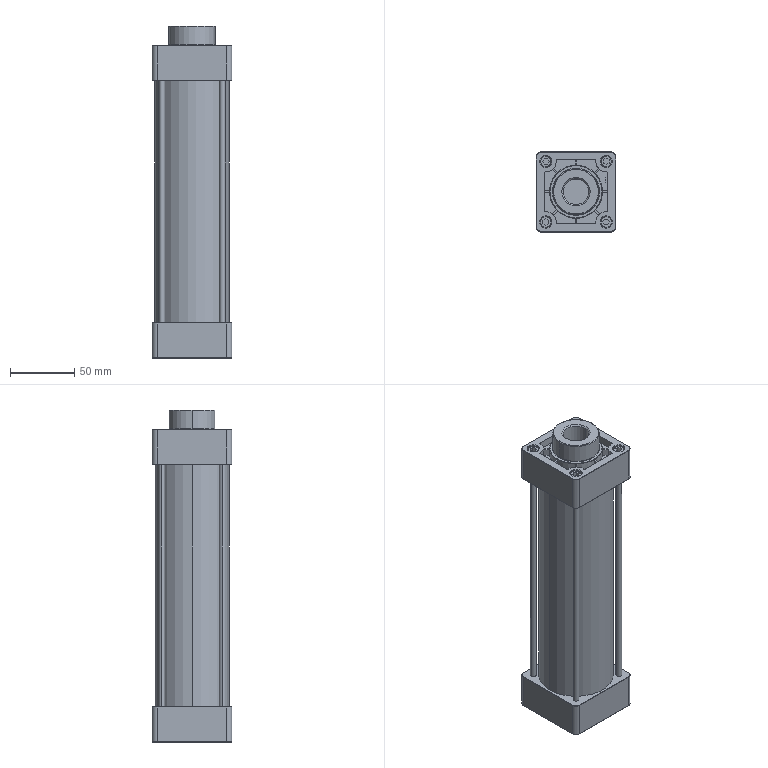Part | SolidWorks | features ICE 11, Fillet 4, Revolution 4, MirrorPattern 3, Chamfer 2, CirPattern 2, Helix 1, RevCut 1, SweepCut 1 | 2 solids | 614 faces | box 62 x 62 x 258 mm | volume 343374 mm3 | plane 296 | spline 136 | cylinder 112 | cone 44 | torus 26 | commonest cylinder face diameters 12.301 x30 8.6 x16 9 x16 2 x10 4.5 x8 8 x8